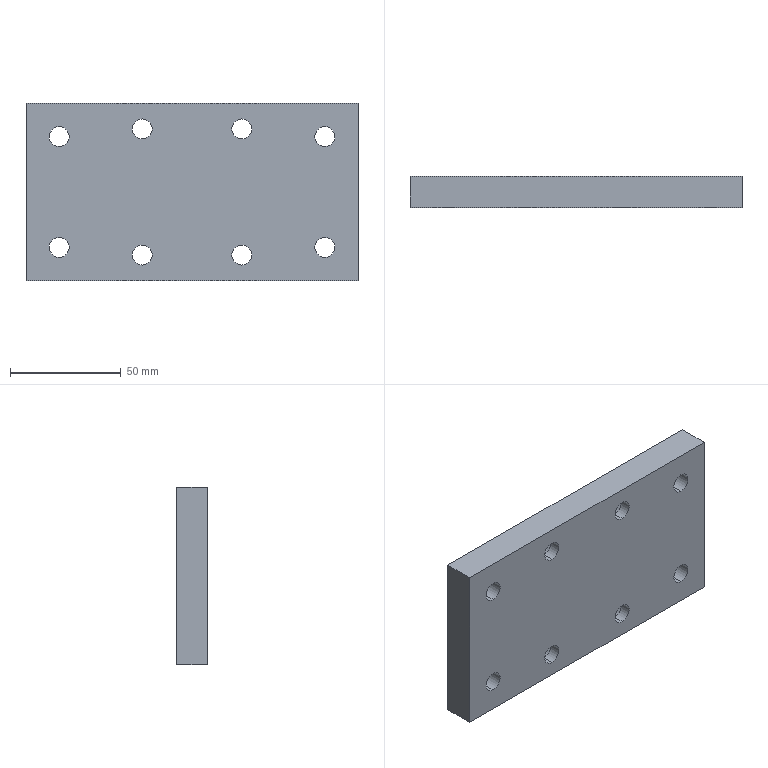Part | SolidWorks | features HoleWzd 2, Extrusion 1 | 1 solid | 34 faces | box 150 x 14 x 80 mm | volume 156803 mm3 | cylinder 24 | plane 10 | commonest cylinder face diameters 9 x16 15 x8
STEP:
#1=CARTESIAN_POINT('',(15.,0.,-69.5));
#2=VERTEX_POINT('',#1);
#3=CARTESIAN_POINT('',(15.,0.,-60.5));
#4=VERTEX_POINT('',#3);
#5=CARTESIAN_POINT('',(15.,0.,-65.));
#6=DIRECTION('',(0.,1.,0.));
#7=DIRECTION('',(0.,0.,1.));
#8=AXIS2_PLACEMENT_3D('',#5,#6,#7);
#9=CIRCLE('',#8,4.5);
#10=EDGE_CURVE('',#2,#4,#9,.T.);
#11=ORIENTED_EDGE('',*,*,#10,.F.);
#12=CARTESIAN_POINT('',(15.,14.,-69.5));
#13=VERTEX_POINT('',#12);
#14=CARTESIAN_POINT('',(15.,14.,-69.5));
#15=DIRECTION('',(0.,1.,0.));
#16=VECTOR('',#15,1000.);
#17=LINE('',#14,#16);
#18=EDGE_CURVE('',#2,#13,#17,.T.);
#19=ORIENTED_EDGE('',*,*,#18,.T.);
#20=CARTESIAN_POINT('',(15.,14.,-60.5));
#21=VERTEX_POINT('',#20);
#22=CARTESIAN_POINT('',(15.,14.,-65.));
#23=DIRECTION('',(0.,1.,0.));
#24=DIRECTION('',(0.,0.,1.));
#25=AXIS2_PLACEMENT_3D('',#22,#23,#24);
#26=CIRCLE('',#25,4.5);
#27=EDGE_CURVE('',#13,#21,#26,.T.);
#28=ORIENTED_EDGE('',*,*,#27,.T.);
#29=CARTESIAN_POINT('',(15.,14.,-60.5));
#30=DIRECTION('',(0.,1.,0.));
#31=VECTOR('',#30,1000.);
#32=LINE('',#29,#31);
#33=EDGE_CURVE('',#4,#21,#32,.T.);
#34=ORIENTED_EDGE('',*,*,#33,.F.);
#35=EDGE_LOOP('',(#11,#19,#28,#34));
#36=FACE_OUTER_BOUND('',#35,.T.);
#37=CARTESIAN_POINT('',(15.,14.,-65.));
#38=DIRECTION('',(0.,1.,0.));
#39=DIRECTION('',(0.,0.,1.));
#40=AXIS2_PLACEMENT_3D('',#37,#38,#39);
#41=CYLINDRICAL_SURFACE('',#40,4.5);
#42=ADVANCED_FACE('',(#36),#41,.F.);
#43=CARTESIAN_POINT('',(15.,0.,-19.5));
#44=VERTEX_POINT('',#43);
#45=CARTESIAN_POINT('',(15.,0.,-10.5));
#46=VERTEX_POINT('',#45);
#47=CARTESIAN_POINT('',(15.,0.,-15.));
#48=DIRECTION('',(0.,1.,0.));
#49=DIRECTION('',(0.,0.,1.));
#50=AXIS2_PLACEMENT_3D('',#47,#48,#49);
#51=CIRCLE('',#50,4.5);
#52=EDGE_CURVE('',#44,#46,#51,.T.);
#53=ORIENTED_EDGE('',*,*,#52,.F.);
#54=CARTESIAN_POINT('',(15.,14.,-19.5));
#55=VERTEX_POINT('',#54);
#56=CARTESIAN_POINT('',(15.,14.,-19.5));
#57=DIRECTION('',(0.,1.,0.));
#58=VECTOR('',#57,1000.);
#59=LINE('',#56,#58);
#60=EDGE_CURVE('',#44,#55,#59,.T.);
#61=ORIENTED_EDGE('',*,*,#60,.T.);
#62=CARTESIAN_POINT('',(15.,14.,-10.5));
#63=VERTEX_POINT('',#62);
#64=CARTESIAN_POINT('',(15.,14.,-15.));
#65=DIRECTION('',(0.,1.,0.));
#66=DIRECTION('',(0.,0.,1.));
#67=AXIS2_PLACEMENT_3D('',#64,#65,#66);
#68=CIRCLE('',#67,4.5);
#69=EDGE_CURVE('',#55,#63,#68,.T.);
#70=ORIENTED_EDGE('',*,*,#69,.T.);
#71=CARTESIAN_POINT('',(15.,14.,-10.5));
#72=DIRECTION('',(0.,1.,0.));
#73=VECTOR('',#72,1000.);
#74=LINE('',#71,#73);
#75=EDGE_CURVE('',#46,#63,#74,.T.);
#76=ORIENTED_EDGE('',*,*,#75,.F.);
#77=EDGE_LOOP('',(#53,#61,#70,#76));
#78=FACE_OUTER_BOUND('',#77,.T.);
#79=CARTESIAN_POINT('',(15.,14.,-15.));
#80=DIRECTION('',(0.,1.,0.));
#81=DIRECTION('',(0.,0.,1.));
#82=AXIS2_PLACEMENT_3D('',#79,#80,#81);
#83=CYLINDRICAL_SURFACE('',#82,4.5);
#84=ADVANCED_FACE('',(#78),#83,.F.);
#85=CARTESIAN_POINT('',(135.,0.,-19.5));
#86=VERTEX_POINT('',#85);
#87=CARTESIAN_POINT('',(135.,0.,-10.5));
#88=VERTEX_POINT('',#87);
#89=CARTESIAN_POINT('',(135.,0.,-15.));
#90=DIRECTION('',(0.,1.,0.));
#91=DIRECTION('',(0.,0.,1.));
#92=AXIS2_PLACEMENT_3D('',#89,#90,#91);
#93=CIRCLE('',#92,4.5);
#94=EDGE_CURVE('',#86,#88,#93,.T.);
#95=ORIENTED_EDGE('',*,*,#94,.F.);
#96=CARTESIAN_POINT('',(135.,14.,-19.5));
#97=VERTEX_POINT('',#96);
#98=CARTESIAN_POINT('',(135.,14.,-19.5));
#99=DIRECTION('',(0.,1.,0.));
#100=VECTOR('',#99,1000.);
#101=LINE('',#98,#100);
#102=EDGE_CURVE('',#86,#97,#101,.T.);
#103=ORIENTED_EDGE('',*,*,#102,.T.);
#104=CARTESIAN_POINT('',(135.,14.,-10.5));
#105=VERTEX_POINT('',#104);
#106=CARTESIAN_POINT('',(135.,14.,-15.));
#107=DIRECTION('',(0.,1.,0.));
#108=DIRECTION('',(0.,0.,1.));
#109=AXIS2_PLACEMENT_3D('',#106,#107,#108);
#110=CIRCLE('',#109,4.5);
#111=EDGE_CURVE('',#97,#105,#110,.T.);
#112=ORIENTED_EDGE('',*,*,#111,.T.);
#113=CARTESIAN_POINT('',(135.,14.,-10.5));
#114=DIRECTION('',(0.,1.,0.));
#115=VECTOR('',#114,1000.);
#116=LINE('',#113,#115);
#117=EDGE_CURVE('',#88,#105,#116,.T.);
#118=ORIENTED_EDGE('',*,*,#117,.F.);
#119=EDGE_LOOP('',(#95,#103,#112,#118));
#120=FACE_OUTER_BOUND('',#119,.T.);
#121=CARTESIAN_POINT('',(135.,14.,-15.));
#122=DIRECTION('',(0.,1.,0.));
#123=DIRECTION('',(0.,0.,1.));
#124=AXIS2_PLACEMENT_3D('',#121,#122,#123);
#125=CYLINDRICAL_SURFACE('',#124,4.5);
#126=ADVANCED_FACE('',(#120),#125,.F.);
#127=CARTESIAN_POINT('',(135.,0.,-69.5));
#128=VERTEX_POINT('',#127);
#129=CARTESIAN_POINT('',(135.,0.,-60.5));
#130=VERTEX_POINT('',#129);
#131=CARTESIAN_POINT('',(135.,0.,-65.));
#132=DIRECTION('',(0.,1.,0.));
#133=DIRECTION('',(0.,0.,1.));
#134=AXIS2_PLACEMENT_3D('',#131,#132,#133);
#135=CIRCLE('',#134,4.5);
#136=EDGE_CURVE('',#128,#130,#135,.T.);
#137=ORIENTED_EDGE('',*,*,#136,.F.);
#138=CARTESIAN_POINT('',(135.,14.,-69.5));
#139=VERTEX_POINT('',#138);
#140=CARTESIAN_POINT('',(135.,14.,-69.5));
#141=DIRECTION('',(0.,1.,0.));
#142=VECTOR('',#141,1000.);
#143=LINE('',#140,#142);
#144=EDGE_CURVE('',#128,#139,#143,.T.);
#145=ORIENTED_EDGE('',*,*,#144,.T.);
#146=CARTESIAN_POINT('',(135.,14.,-60.5));
#147=VERTEX_POINT('',#146);
#148=CARTESIAN_POINT('',(135.,14.,-65.));
#149=DIRECTION('',(0.,1.,0.));
#150=DIRECTION('',(0.,0.,1.));
#151=AXIS2_PLACEMENT_3D('',#148,#149,#150);
#152=CIRCLE('',#151,4.5);
#153=EDGE_CURVE('',#139,#147,#152,.T.);
#154=ORIENTED_EDGE('',*,*,#153,.T.);
#155=CARTESIAN_POINT('',(135.,14.,-60.5));
#156=DIRECTION('',(0.,1.,0.));
#157=VECTOR('',#156,1000.);
#158=LINE('',#155,#157);
#159=EDGE_CURVE('',#130,#147,#158,.T.);
#160=ORIENTED_EDGE('',*,*,#159,.F.);
#161=EDGE_LOOP('',(#137,#145,#154,#160));
#162=FACE_OUTER_BOUND('',#161,.T.);
#163=CARTESIAN_POINT('',(135.,14.,-65.));
#164=DIRECTION('',(0.,1.,0.));
#165=DIRECTION('',(0.,0.,1.));
#166=AXIS2_PLACEMENT_3D('',#163,#164,#165);
#167=CYLINDRICAL_SURFACE('',#166,4.5);
#168=ADVANCED_FACE('',(#162),#167,.F.);
#169=CARTESIAN_POINT('',(52.5,5.,-76.));
#170=VERTEX_POINT('',#169);
#171=CARTESIAN_POINT('',(52.5,5.,-61.));
#172=VERTEX_POINT('',#171);
#173=CARTESIAN_POINT('',(52.5,5.,-68.5));
#174=DIRECTION('',(0.,1.,0.));
#175=DIRECTION('',(0.,0.,1.));
#176=AXIS2_PLACEMENT_3D('',#173,#174,#175);
#177=CIRCLE('',#176,7.5);
#178=EDGE_CURVE('',#170,#172,#177,.T.);
#179=ORIENTED_EDGE('',*,*,#178,.F.);
#180=CARTESIAN_POINT('',(52.5,14.,-76.));
#181=VERTEX_POINT('',#180);
#182=CARTESIAN_POINT('',(52.5,14.,-76.));
#183=DIRECTION('',(0.,1.,0.));
#184=VECTOR('',#183,1000.);
#185=LINE('',#182,#184);
#186=EDGE_CURVE('',#170,#181,#185,.T.);
#187=ORIENTED_EDGE('',*,*,#186,.T.);
#188=CARTESIAN_POINT('',(52.5,14.,-61.));
#189=VERTEX_POINT('',#188);
#190=CARTESIAN_POINT('',(52.5,14.,-68.5));
#191=DIRECTION('',(0.,1.,0.));
#192=DIRECTION('',(0.,0.,1.));
#193=AXIS2_PLACEMENT_3D('',#190,#191,#192);
#194=CIRCLE('',#193,7.5);
#195=EDGE_CURVE('',#181,#189,#194,.T.);
#196=ORIENTED_EDGE('',*,*,#195,.T.);
#197=CARTESIAN_POINT('',(52.5,14.,-61.));
#198=DIRECTION('',(0.,1.,0.));
#199=VECTOR('',#198,1000.);
#200=LINE('',#197,#199);
#201=EDGE_CURVE('',#172,#189,#200,.T.);
#202=ORIENTED_EDGE('',*,*,#201,.F.);
#203=EDGE_LOOP('',(#179,#187,#196,#202));
#204=FACE_OUTER_BOUND('',#203,.T.);
#205=CARTESIAN_POINT('',(52.5,14.,-68.5));
#206=DIRECTION('',(0.,1.,0.));
#207=DIRECTION('',(0.,0.,1.));
#208=AXIS2_PLACEMENT_3D('',#205,#206,#207);
#209=CYLINDRICAL_SURFACE('',#208,7.5);
#210=ADVANCED_FACE('',(#204),#209,.F.);
#211=CARTESIAN_POINT('',(52.5,0.,-73.));
#212=VERTEX_POINT('',#211);
#213=CARTESIAN_POINT('',(52.5,0.,-64.));
#214=VERTEX_POINT('',#213);
#215=CARTESIAN_POINT('',(52.5,0.,-68.5));
#216=DIRECTION('',(0.,1.,0.));
#217=DIRECTION('',(0.,0.,1.));
#218=AXIS2_PLACEMENT_3D('',#215,#216,#217);
#219=CIRCLE('',#218,4.5);
#220=EDGE_CURVE('',#212,#214,#219,.T.);
#221=ORIENTED_EDGE('',*,*,#220,.F.);
#222=CARTESIAN_POINT('',(52.5,5.,-73.));
#223=VERTEX_POINT('',#222);
#224=CARTESIAN_POINT('',(52.5,14.,-73.));
#225=DIRECTION('',(0.,1.,0.));
#226=VECTOR('',#225,1000.);
#227=LINE('',#224,#226);
#228=EDGE_CURVE('',#212,#223,#227,.T.);
#229=ORIENTED_EDGE('',*,*,#228,.T.);
#230=CARTESIAN_POINT('',(52.5,5.,-64.));
#231=VERTEX_POINT('',#230);
#232=CARTESIAN_POINT('',(52.5,5.,-68.5));
#233=DIRECTION('',(0.,1.,0.));
#234=DIRECTION('',(0.,0.,1.));
#235=AXIS2_PLACEMENT_3D('',#232,#233,#234);
#236=CIRCLE('',#235,4.5);
#237=EDGE_CURVE('',#223,#231,#236,.T.);
#238=ORIENTED_EDGE('',*,*,#237,.T.);
#239=CARTESIAN_POINT('',(52.5,14.,-64.));
#240=DIRECTION('',(0.,1.,0.));
#241=VECTOR('',#240,1000.);
#242=LINE('',#239,#241);
#243=EDGE_CURVE('',#214,#231,#242,.T.);
#244=ORIENTED_EDGE('',*,*,#243,.F.);
#245=EDGE_LOOP('',(#221,#229,#238,#244));
#246=FACE_OUTER_BOUND('',#245,.T.);
#247=CARTESIAN_POINT('',(52.5,14.,-68.5));
#248=DIRECTION('',(0.,1.,0.));
#249=DIRECTION('',(0.,0.,1.));
#250=AXIS2_PLACEMENT_3D('',#247,#248,#249);
#251=CYLINDRICAL_SURFACE('',#250,4.5);
#252=ADVANCED_FACE('',(#246),#251,.F.);
#253=CARTESIAN_POINT('',(52.5,5.,-19.));
#254=VERTEX_POINT('',#253);
#255=CARTESIAN_POINT('',(52.5,5.,-4.));
#256=VERTEX_POINT('',#255);
#257=CARTESIAN_POINT('',(52.5,5.,-11.5));
#258=DIRECTION('',(0.,1.,0.));
#259=DIRECTION('',(0.,0.,1.));
#260=AXIS2_PLACEMENT_3D('',#257,#258,#259);
#261=CIRCLE('',#260,7.5);
#262=EDGE_CURVE('',#254,#256,#261,.T.);
#263=ORIENTED_EDGE('',*,*,#262,.F.);
#264=CARTESIAN_POINT('',(52.5,14.,-19.));
#265=VERTEX_POINT('',#264);
#266=CARTESIAN_POINT('',(52.5,14.,-19.));
#267=DIRECTION('',(0.,1.,0.));
#268=VECTOR('',#267,1000.);
#269=LINE('',#266,#268);
#270=EDGE_CURVE('',#254,#265,#269,.T.);
#271=ORIENTED_EDGE('',*,*,#270,.T.);
#272=CARTESIAN_POINT('',(52.5,14.,-4.));
#273=VERTEX_POINT('',#272);
#274=CARTESIAN_POINT('',(52.5,14.,-11.5));
#275=DIRECTION('',(0.,1.,0.));
#276=DIRECTION('',(0.,0.,1.));
#277=AXIS2_PLACEMENT_3D('',#274,#275,#276);
#278=CIRCLE('',#277,7.5);
#279=EDGE_CURVE('',#265,#273,#278,.T.);
#280=ORIENTED_EDGE('',*,*,#279,.T.);
#281=CARTESIAN_POINT('',(52.5,14.,-4.));
#282=DIRECTION('',(0.,1.,0.));
#283=VECTOR('',#282,1000.);
#284=LINE('',#281,#283);
#285=EDGE_CURVE('',#256,#273,#284,.T.);
#286=ORIENTED_EDGE('',*,*,#285,.F.);
#287=EDGE_LOOP('',(#263,#271,#280,#286));
#288=FACE_OUTER_BOUND('',#287,.T.);
#289=CARTESIAN_POINT('',(52.5,14.,-11.5));
#290=DIRECTION('',(0.,1.,0.));
#291=DIRECTION('',(0.,0.,1.));
#292=AXIS2_PLACEMENT_3D('',#289,#290,#291);
#293=CYLINDRICAL_SURFACE('',#292,7.5);
#294=ADVANCED_FACE('',(#288),#293,.F.);
#295=CARTESIAN_POINT('',(52.5,0.,-16.));
#296=VERTEX_POINT('',#295);
#297=CARTESIAN_POINT('',(52.5,0.,-7.));
#298=VERTEX_POINT('',#297);
#299=CARTESIAN_POINT('',(52.5,0.,-11.5));
#300=DIRECTION('',(0.,1.,0.));
#301=DIRECTION('',(0.,0.,1.));
#302=AXIS2_PLACEMENT_3D('',#299,#300,#301);
#303=CIRCLE('',#302,4.5);
#304=EDGE_CURVE('',#296,#298,#303,.T.);
#305=ORIENTED_EDGE('',*,*,#304,.F.);
#306=CARTESIAN_POINT('',(52.5,5.,-16.));
#307=VERTEX_POINT('',#306);
#308=CARTESIAN_POINT('',(52.5,14.,-16.));
#309=DIRECTION('',(0.,1.,0.));
#310=VECTOR('',#309,1000.);
#311=LINE('',#308,#310);
#312=EDGE_CURVE('',#296,#307,#311,.T.);
#313=ORIENTED_EDGE('',*,*,#312,.T.);
#314=CARTESIAN_POINT('',(52.5,5.,-7.));
#315=VERTEX_POINT('',#314);
#316=CARTESIAN_POINT('',(52.5,5.,-11.5));
#317=DIRECTION('',(0.,1.,0.));
#318=DIRECTION('',(0.,0.,1.));
#319=AXIS2_PLACEMENT_3D('',#316,#317,#318);
#320=CIRCLE('',#319,4.5);
#321=EDGE_CURVE('',#307,#315,#320,.T.);
#322=ORIENTED_EDGE('',*,*,#321,.T.);
#323=CARTESIAN_POINT('',(52.5,14.,-7.));
#324=DIRECTION('',(0.,1.,0.));
#325=VECTOR('',#324,1000.);
#326=LINE('',#323,#325);
#327=EDGE_CURVE('',#298,#315,#326,.T.);
#328=ORIENTED_EDGE('',*,*,#327,.F.);
#329=EDGE_LOOP('',(#305,#313,#322,#328));
#330=FACE_OUTER_BOUND('',#329,.T.);
#331=CARTESIAN_POINT('',(52.5,14.,-11.5));
#332=DIRECTION('',(0.,1.,0.));
#333=DIRECTION('',(0.,0.,1.));
#334=AXIS2_PLACEMENT_3D('',#331,#332,#333);
#335=CYLINDRICAL_SURFACE('',#334,4.5);
#336=ADVANCED_FACE('',(#330),#335,.F.);
#337=CARTESIAN_POINT('',(97.5,5.,-19.));
#338=VERTEX_POINT('',#337);
#339=CARTESIAN_POINT('',(97.5,5.,-4.));
#340=VERTEX_POINT('',#339);
#341=CARTESIAN_POINT('',(97.5,5.,-11.5));
#342=DIRECTION('',(0.,1.,0.));
#343=DIRECTION('',(0.,0.,1.));
#344=AXIS2_PLACEMENT_3D('',#341,#342,#343);
#345=CIRCLE('',#344,7.5);
#346=EDGE_CURVE('',#338,#340,#345,.T.);
#347=ORIENTED_EDGE('',*,*,#346,.F.);
#348=CARTESIAN_POINT('',(97.5,14.,-19.));
#349=VERTEX_POINT('',#348);
#350=CARTESIAN_POINT('',(97.5,14.,-19.));
#351=DIRECTION('',(0.,1.,0.));
#352=VECTOR('',#351,1000.);
#353=LINE('',#350,#352);
#354=EDGE_CURVE('',#338,#349,#353,.T.);
#355=ORIENTED_EDGE('',*,*,#354,.T.);
#356=CARTESIAN_POINT('',(97.5,14.,-4.));
#357=VERTEX_POINT('',#356);
#358=CARTESIAN_POINT('',(97.5,14.,-11.5));
#359=DIRECTION('',(0.,1.,0.));
#360=DIRECTION('',(0.,0.,1.));
#361=AXIS2_PLACEMENT_3D('',#358,#359,#360);
#362=CIRCLE('',#361,7.5);
#363=EDGE_CURVE('',#349,#357,#362,.T.);
#364=ORIENTED_EDGE('',*,*,#363,.T.);
#365=CARTESIAN_POINT('',(97.5,14.,-4.));
#366=DIRECTION('',(0.,1.,0.));
#367=VECTOR('',#366,1000.);
#368=LINE('',#365,#367);
#369=EDGE_CURVE('',#340,#357,#368,.T.);
#370=ORIENTED_EDGE('',*,*,#369,.F.);
#371=EDGE_LOOP('',(#347,#355,#364,#370));
#372=FACE_OUTER_BOUND('',#371,.T.);
#373=CARTESIAN_POINT('',(97.5,14.,-11.5));
#374=DIRECTION('',(0.,1.,0.));
#375=DIRECTION('',(0.,0.,1.));
#376=AXIS2_PLACEMENT_3D('',#373,#374,#375);
#377=CYLINDRICAL_SURFACE('',#376,7.5);
#378=ADVANCED_FACE('',(#372),#377,.F.);
#379=CARTESIAN_POINT('',(97.5,0.,-16.));
#380=VERTEX_POINT('',#379);
#381=CARTESIAN_POINT('',(97.5,0.,-7.));
#382=VERTEX_POINT('',#381);
#383=CARTESIAN_POINT('',(97.5,0.,-11.5));
#384=DIRECTION('',(0.,1.,0.));
#385=DIRECTION('',(0.,0.,1.));
#386=AXIS2_PLACEMENT_3D('',#383,#384,#385);
#387=CIRCLE('',#386,4.5);
#388=EDGE_CURVE('',#380,#382,#387,.T.);
#389=ORIENTED_EDGE('',*,*,#388,.F.);
#390=CARTESIAN_POINT('',(97.5,5.,-16.));
#391=VERTEX_POINT('',#390);
#392=CARTESIAN_POINT('',(97.5,14.,-16.));
#393=DIRECTION('',(0.,1.,0.));
#394=VECTOR('',#393,1000.);
#395=LINE('',#392,#394);
#396=EDGE_CURVE('',#380,#391,#395,.T.);
#397=ORIENTED_EDGE('',*,*,#396,.T.);
#398=CARTESIAN_POINT('',(97.5,5.,-7.));
#399=VERTEX_POINT('',#398);
#400=CARTESIAN_POINT('',(97.5,5.,-11.5));
#401=DIRECTION('',(0.,1.,0.));
#402=DIRECTION('',(0.,0.,1.));
#403=AXIS2_PLACEMENT_3D('',#400,#401,#402);
#404=CIRCLE('',#403,4.5);
#405=EDGE_CURVE('',#391,#399,#404,.T.);
#406=ORIENTED_EDGE('',*,*,#405,.T.);
#407=CARTESIAN_POINT('',(97.5,14.,-7.));
#408=DIRECTION('',(0.,1.,0.));
#409=VECTOR('',#408,1000.);
#410=LINE('',#407,#409);
#411=EDGE_CURVE('',#382,#399,#410,.T.);
#412=ORIENTED_EDGE('',*,*,#411,.F.);
#413=EDGE_LOOP('',(#389,#397,#406,#412));
#414=FACE_OUTER_BOUND('',#413,.T.);
#415=CARTESIAN_POINT('',(97.5,14.,-11.5));
#416=DIRECTION('',(0.,1.,0.));
#417=DIRECTION('',(0.,0.,1.));
#418=AXIS2_PLACEMENT_3D('',#415,#416,#417);
#419=CYLINDRICAL_SURFACE('',#418,4.5);
#420=ADVANCED_FACE('',(#414),#419,.F.);
#421=CARTESIAN_POINT('',(97.5,5.,-76.));
#422=VERTEX_POINT('',#421);
#423=CARTESIAN_POINT('',(97.5,5.,-61.));
#424=VERTEX_POINT('',#423);
#425=CARTESIAN_POINT('',(97.5,5.,-68.5));
#426=DIRECTION('',(0.,1.,0.));
#427=DIRECTION('',(0.,0.,1.));
#428=AXIS2_PLACEMENT_3D('',#425,#426,#427);
#429=CIRCLE('',#428,7.5);
#430=EDGE_CURVE('',#422,#424,#429,.T.);
#431=ORIENTED_EDGE('',*,*,#430,.F.);
#432=CARTESIAN_POINT('',(97.5,14.,-76.));
#433=VERTEX_POINT('',#432);
#434=CARTESIAN_POINT('',(97.5,14.,-76.));
#435=DIRECTION('',(0.,1.,0.));
#436=VECTOR('',#435,1000.);
#437=LINE('',#434,#436);
#438=EDGE_CURVE('',#422,#433,#437,.T.);
#439=ORIENTED_EDGE('',*,*,#438,.T.);
#440=CARTESIAN_POINT('',(97.5,14.,-61.));
#441=VERTEX_POINT('',#440);
#442=CARTESIAN_POINT('',(97.5,14.,-68.5));
#443=DIRECTION('',(0.,1.,0.));
#444=DIRECTION('',(0.,0.,1.));
#445=AXIS2_PLACEMENT_3D('',#442,#443,#444);
#446=CIRCLE('',#445,7.5);
#447=EDGE_CURVE('',#433,#441,#446,.T.);
#448=ORIENTED_EDGE('',*,*,#447,.T.);
#449=CARTESIAN_POINT('',(97.5,14.,-61.));
#450=DIRECTION('',(0.,1.,0.));
#451=VECTOR('',#450,1000.);
#452=LINE('',#449,#451);
#453=EDGE_CURVE('',#424,#441,#452,.T.);
#454=ORIENTED_EDGE('',*,*,#453,.F.);
#455=EDGE_LOOP('',(#431,#439,#448,#454));
#456=FACE_OUTER_BOUND('',#455,.T.);
#457=CARTESIAN_POINT('',(97.5,14.,-68.5));
#458=DIRECTION('',(0.,1.,0.));
#459=DIRECTION('',(0.,0.,1.));
#460=AXIS2_PLACEMENT_3D('',#457,#458,#459);
#461=CYLINDRICAL_SURFACE('',#460,7.5);
#462=ADVANCED_FACE('',(#456),#461,.F.);
#463=CARTESIAN_POINT('',(97.5,0.,-73.));
#464=VERTEX_POINT('',#463);
#465=CARTESIAN_POINT('',(97.5,0.,-64.));
#466=VERTEX_POINT('',#465);
#467=CARTESIAN_POINT('',(97.5,0.,-68.5));
#468=DIRECTION('',(0.,1.,0.));
#469=DIRECTION('',(0.,0.,1.));
#470=AXIS2_PLACEMENT_3D('',#467,#468,#469);
#471=CIRCLE('',#470,4.5);
#472=EDGE_CURVE('',#464,#466,#471,.T.);
#473=ORIENTED_EDGE('',*,*,#472,.F.);
#474=CARTESIAN_POINT('',(97.5,5.,-73.));
#475=VERTEX_POINT('',#474);
#476=CARTESIAN_POINT('',(97.5,14.,-73.));
#477=DIRECTION('',(0.,1.,0.));
#478=VECTOR('',#477,1000.);
#479=LINE('',#476,#478);
#480=EDGE_CURVE('',#464,#475,#479,.T.);
#481=ORIENTED_EDGE('',*,*,#480,.T.);
#482=CARTESIAN_POINT('',(97.5,5.,-64.));
#483=VERTEX_POINT('',#482);
#484=CARTESIAN_POINT('',(97.5,5.,-68.5));
#485=DIRECTION('',(0.,1.,0.));
#486=DIRECTION('',(0.,0.,1.));
#487=AXIS2_PLACEMENT_3D('',#484,#485,#486);
#488=CIRCLE('',#487,4.5);
#489=EDGE_CURVE('',#475,#483,#488,.T.);
#490=ORIENTED_EDGE('',*,*,#489,.T.);
#491=CARTESIAN_POINT('',(97.5,14.,-64.));
#492=DIRECTION('',(0.,1.,0.));
#493=VECTOR('',#492,1000.);
#494=LINE('',#491,#493);
#495=EDGE_CURVE('',#466,#483,#494,.T.);
#496=ORIENTED_EDGE('',*,*,#495,.F.);
#497=EDGE_LOOP('',(#473,#481,#490,#496));
#498=FACE_OUTER_BOUND('',#497,.T.);
#499=CARTESIAN_POINT('',(97.5,14.,-68.5));
#500=DIRECTION('',(0.,1.,0.));
#501=DIRECTION('',(0.,0.,1.));
#502=AXIS2_PLACEMENT_3D('',#499,#500,#501);
#503=CYLINDRICAL_SURFACE('',#502,4.5);
#504=ADVANCED_FACE('',(#498),#503,.F.);
#505=CARTESIAN_POINT('',(0.,0.,-80.));
#506=VERTEX_POINT('',#505);
#507=CARTESIAN_POINT('',(0.,0.,0.));
#508=VERTEX_POINT('',#507);
#509=CARTESIAN_POINT('',(0.,0.,0.));
#510=DIRECTION('',(0.,0.,1.));
#511=VECTOR('',#510,1000.);
#512=LINE('',#509,#511);
#513=EDGE_CURVE('',#506,#508,#512,.T.);
#514=ORIENTED_EDGE('',*,*,#513,.T.);
#515=CARTESIAN_POINT('',(0.,14.,0.));
#516=VERTEX_POINT('',#515);
#517=CARTESIAN_POINT('',(0.,14.,0.));
#518=DIRECTION('',(0.,-1.,0.));
#519=VECTOR('',#518,1000.);
#520=LINE('',#517,#519);
#521=EDGE_CURVE('',#516,#508,#520,.T.);
#522=ORIENTED_EDGE('',*,*,#521,.F.);
#523=CARTESIAN_POINT('',(0.,14.,-80.));
#524=VERTEX_POINT('',#523);
#525=CARTESIAN_POINT('',(0.,14.,0.));
#526=DIRECTION('',(0.,0.,1.));
#527=VECTOR('',#526,1000.);
#528=LINE('',#525,#527);
#529=EDGE_CURVE('',#524,#516,#528,.T.);
#530=ORIENTED_EDGE('',*,*,#529,.F.);
#531=CARTESIAN_POINT('',(0.,14.,-80.));
#532=DIRECTION('',(0.,-1.,0.));
#533=VECTOR('',#532,1000.);
#534=LINE('',#531,#533);
#535=EDGE_CURVE('',#524,#506,#534,.T.);
#536=ORIENTED_EDGE('',*,*,#535,.T.);
#537=EDGE_LOOP('',(#514,#522,#530,#536));
#538=FACE_OUTER_BOUND('',#537,.T.);
#539=CARTESIAN_POINT('',(0.,14.,0.));
#540=DIRECTION('',(1.,0.,0.));
#541=DIRECTION('',(0.,0.,-1.));
#542=AXIS2_PLACEMENT_3D('',#539,#540,#541);
#543=PLANE('',#542);
#544=ADVANCED_FACE('',(#538),#543,.F.);
#545=CARTESIAN_POINT('',(150.,0.,0.));
#546=VERTEX_POINT('',#545);
#547=CARTESIAN_POINT('',(0.,0.,0.));
#548=DIRECTION('',(1.,0.,0.));
#549=VECTOR('',#548,1000.);
#550=LINE('',#547,#549);
#551=EDGE_CURVE('',#508,#546,#550,.T.);
#552=ORIENTED_EDGE('',*,*,#551,.T.);
#553=CARTESIAN_POINT('',(150.,14.,0.));
#554=VERTEX_POINT('',#553);
#555=CARTESIAN_POINT('',(150.,14.,0.));
#556=DIRECTION('',(0.,-1.,0.));
#557=VECTOR('',#556,1000.);
#558=LINE('',#555,#557);
#559=EDGE_CURVE('',#554,#546,#558,.T.);
#560=ORIENTED_EDGE('',*,*,#559,.F.);
#561=CARTESIAN_POINT('',(0.,14.,0.));
#562=DIRECTION('',(1.,0.,0.));
#563=VECTOR('',#562,1000.);
#564=LINE('',#561,#563);
#565=EDGE_CURVE('',#516,#554,#564,.T.);
#566=ORIENTED_EDGE('',*,*,#565,.F.);
#567=ORIENTED_EDGE('',*,*,#521,.T.);
#568=EDGE_LOOP('',(#552,#560,#566,#567));
#569=FACE_OUTER_BOUND('',#568,.T.);
#570=CARTESIAN_POINT('',(0.,14.,0.));
#571=DIRECTION('',(0.,0.,-1.));
#572=DIRECTION('',(-1.,0.,0.));
#573=AXIS2_PLACEMENT_3D('',#570,#571,#572);
#574=PLANE('',#573);
#575=ADVANCED_FACE('',(#569),#574,.F.);
#576=CARTESIAN_POINT('',(150.,0.,-80.));
#577=VERTEX_POINT('',#576);
#578=CARTESIAN_POINT('',(150.,0.,0.));
#579=DIRECTION('',(0.,0.,-1.));
#580=VECTOR('',#579,1000.);
#581=LINE('',#578,#580);
#582=EDGE_CURVE('',#546,#577,#581,.T.);
#583=ORIENTED_EDGE('',*,*,#582,.T.);
#584=CARTESIAN_POINT('',(150.,14.,-80.));
#585=VERTEX_POINT('',#584);
#586=CARTESIAN_POINT('',(150.,14.,-80.));
#587=DIRECTION('',(0.,-1.,0.));
#588=VECTOR('',#587,1000.);
#589=LINE('',#586,#588);
#590=EDGE_CURVE('',#585,#577,#589,.T.);
#591=ORIENTED_EDGE('',*,*,#590,.F.);
#592=CARTESIAN_POINT('',(150.,14.,0.));
#593=DIRECTION('',(0.,0.,-1.));
#594=VECTOR('',#593,1000.);
#595=LINE('',#592,#594);
#596=EDGE_CURVE('',#554,#585,#595,.T.);
#597=ORIENTED_EDGE('',*,*,#596,.F.);
#598=ORIENTED_EDGE('',*,*,#559,.T.);
#599=EDGE_LOOP('',(#583,#591,#597,#598));
#600=FACE_OUTER_BOUND('',#599,.T.);
#601=CARTESIAN_POINT('',(150.,14.,0.));
#602=DIRECTION('',(-1.,0.,0.));
#603=DIRECTION('',(0.,0.,1.));
#604=AXIS2_PLACEMENT_3D('',#601,#602,#603);
#605=PLANE('',#604);
#606=ADVANCED_FACE('',(#600),#605,.F.);
#607=CARTESIAN_POINT('',(0.,0.,-80.));
#608=DIRECTION('',(-1.,0.,0.));
#609=VECTOR('',#608,1000.);
#610=LINE('',#607,#609);
#611=EDGE_CURVE('',#577,#506,#610,.T.);
#612=ORIENTED_EDGE('',*,*,#611,.T.);
#613=ORIENTED_EDGE('',*,*,#535,.F.);
#614=CARTESIAN_POINT('',(0.,14.,-80.));
#615=DIRECTION('',(-1.,0.,0.));
#616=VECTOR('',#615,1000.);
#617=LINE('',#614,#616);
#618=EDGE_CURVE('',#585,#524,#617,.T.);
#619=ORIENTED_EDGE('',*,*,#618,.F.);
#620=ORIENTED_EDGE('',*,*,#590,.T.);
#621=EDGE_LOOP('',(#612,#613,#619,#620));
#622=FACE_OUTER_BOUND('',#621,.T.);
#623=CARTESIAN_POINT('',(0.,14.,-80.));
#624=DIRECTION('',(0.,0.,1.));
#625=DIRECTION('',(1.,0.,0.));
#626=AXIS2_PLACEMENT_3D('',#623,#624,#625);
#627=PLANE('',#626);
#628=ADVANCED_FACE('',(#622),#627,.F.);
#629=CARTESIAN_POINT('',(15.,14.,-65.));
#630=DIRECTION('',(0.,1.,0.));
#631=DIRECTION('',(0.,0.,1.));
#632=AXIS2_PLACEMENT_3D('',#629,#630,#631);
#633=CIRCLE('',#632,4.5);
#634=EDGE_CURVE('',#21,#13,#633,.T.);
#635=ORIENTED_EDGE('',*,*,#634,.F.);
#636=ORIENTED_EDGE('',*,*,#27,.F.);
#637=EDGE_LOOP('',(#635,#636));
#638=FACE_BOUND('',#637,.T.);
#639=CARTESIAN_POINT('',(15.,14.,-15.));
#640=DIRECTION('',(0.,1.,0.));
#641=DIRECTION('',(0.,0.,1.));
#642=AXIS2_PLACEMENT_3D('',#639,#640,#641);
#643=CIRCLE('',#642,4.5);
#644=EDGE_CURVE('',#63,#55,#643,.T.);
#645=ORIENTED_EDGE('',*,*,#644,.F.);
#646=ORIENTED_EDGE('',*,*,#69,.F.);
#647=EDGE_LOOP('',(#645,#646));
#648=FACE_BOUND('',#647,.T.);
#649=CARTESIAN_POINT('',(135.,14.,-15.));
#650=DIRECTION('',(0.,1.,0.));
#651=DIRECTION('',(0.,0.,1.));
#652=AXIS2_PLACEMENT_3D('',#649,#650,#651);
#653=CIRCLE('',#652,4.5);
#654=EDGE_CURVE('',#105,#97,#653,.T.);
#655=ORIENTED_EDGE('',*,*,#654,.F.);
#656=ORIENTED_EDGE('',*,*,#111,.F.);
#657=EDGE_LOOP('',(#655,#656));
#658=FACE_BOUND('',#657,.T.);
#659=CARTESIAN_POINT('',(135.,14.,-65.));
#660=DIRECTION('',(0.,1.,0.));
#661=DIRECTION('',(0.,0.,1.));
#662=AXIS2_PLACEMENT_3D('',#659,#660,#661);
#663=CIRCLE('',#662,4.5);
#664=EDGE_CURVE('',#147,#139,#663,.T.);
#665=ORIENTED_EDGE('',*,*,#664,.F.);
#666=ORIENTED_EDGE('',*,*,#153,.F.);
#667=EDGE_LOOP('',(#665,#666));
#668=FACE_BOUND('',#667,.T.);
#669=CARTESIAN_POINT('',(52.5,14.,-68.5));
#670=DIRECTION('',(0.,1.,0.));
#671=DIRECTION('',(0.,0.,1.));
#672=AXIS2_PLACEMENT_3D('',#669,#670,#671);
#673=CIRCLE('',#672,7.5);
#674=EDGE_CURVE('',#189,#181,#673,.T.);
#675=ORIENTED_EDGE('',*,*,#674,.F.);
#676=ORIENTED_EDGE('',*,*,#195,.F.);
#677=EDGE_LOOP('',(#675,#676));
#678=FACE_BOUND('',#677,.T.);
#679=CARTESIAN_POINT('',(52.5,14.,-11.5));
#680=DIRECTION('',(0.,1.,0.));
#681=DIRECTION('',(0.,0.,1.));
#682=AXIS2_PLACEMENT_3D('',#679,#680,#681);
#683=CIRCLE('',#682,7.5);
#684=EDGE_CURVE('',#273,#265,#683,.T.);
#685=ORIENTED_EDGE('',*,*,#684,.F.);
#686=ORIENTED_EDGE('',*,*,#279,.F.);
#687=EDGE_LOOP('',(#685,#686));
#688=FACE_BOUND('',#687,.T.);
#689=CARTESIAN_POINT('',(97.5,14.,-11.5));
#690=DIRECTION('',(0.,1.,0.));
#691=DIRECTION('',(0.,0.,1.));
#692=AXIS2_PLACEMENT_3D('',#689,#690,#691);
#693=CIRCLE('',#692,7.5);
#694=EDGE_CURVE('',#357,#349,#693,.T.);
#695=ORIENTED_EDGE('',*,*,#694,.F.);
#696=ORIENTED_EDGE('',*,*,#363,.F.);
#697=EDGE_LOOP('',(#695,#696));
#698=FACE_BOUND('',#697,.T.);
#699=CARTESIAN_POINT('',(97.5,14.,-68.5));
#700=DIRECTION('',(0.,1.,0.));
#701=DIRECTION('',(0.,0.,1.));
#702=AXIS2_PLACEMENT_3D('',#699,#700,#701);
#703=CIRCLE('',#702,7.5);
#704=EDGE_CURVE('',#441,#433,#703,.T.);
#705=ORIENTED_EDGE('',*,*,#704,.F.);
#706=ORIENTED_EDGE('',*,*,#447,.F.);
#707=EDGE_LOOP('',(#705,#706));
#708=FACE_BOUND('',#707,.T.);
#709=ORIENTED_EDGE('',*,*,#529,.T.);
#710=ORIENTED_EDGE('',*,*,#565,.T.);
#711=ORIENTED_EDGE('',*,*,#596,.T.);
#712=ORIENTED_EDGE('',*,*,#618,.T.);
#713=EDGE_LOOP('',(#709,#710,#711,#712));
#714=FACE_OUTER_BOUND('',#713,.T.);
#715=CARTESIAN_POINT('',(0.,14.,0.));
#716=DIRECTION('',(0.,-1.,0.));
#717=DIRECTION('',(0.,0.,-1.));
#718=AXIS2_PLACEMENT_3D('',#715,#716,#717);
#719=PLANE('',#718);
#720=ADVANCED_FACE('',(#638,#648,#658,#668,#678,#688,#698,#708,#714),#719,.F.);
#721=CARTESIAN_POINT('',(15.,0.,-65.));
#722=DIRECTION('',(0.,1.,0.));
#723=DIRECTION('',(0.,0.,1.));
#724=AXIS2_PLACEMENT_3D('',#721,#722,#723);
#725=CIRCLE('',#724,4.5);
#726=EDGE_CURVE('',#4,#2,#725,.T.);
#727=ORIENTED_EDGE('',*,*,#726,.T.);
#728=ORIENTED_EDGE('',*,*,#10,.T.);
#729=EDGE_LOOP('',(#727,#728));
#730=FACE_BOUND('',#729,.T.);
#731=CARTESIAN_POINT('',(15.,0.,-15.));
#732=DIRECTION('',(0.,1.,0.));
#733=DIRECTION('',(0.,0.,1.));
#734=AXIS2_PLACEMENT_3D('',#731,#732,#733);
#735=CIRCLE('',#734,4.5);
#736=EDGE_CURVE('',#46,#44,#735,.T.);
#737=ORIENTED_EDGE('',*,*,#736,.T.);
#738=ORIENTED_EDGE('',*,*,#52,.T.);
#739=EDGE_LOOP('',(#737,#738));
#740=FACE_BOUND('',#739,.T.);
#741=CARTESIAN_POINT('',(135.,0.,-15.));
#742=DIRECTION('',(0.,1.,0.));
#743=DIRECTION('',(0.,0.,1.));
#744=AXIS2_PLACEMENT_3D('',#741,#742,#743);
#745=CIRCLE('',#744,4.5);
#746=EDGE_CURVE('',#88,#86,#745,.T.);
#747=ORIENTED_EDGE('',*,*,#746,.T.);
#748=ORIENTED_EDGE('',*,*,#94,.T.);
#749=EDGE_LOOP('',(#747,#748));
#750=FACE_BOUND('',#749,.T.);
#751=CARTESIAN_POINT('',(135.,0.,-65.));
#752=DIRECTION('',(0.,1.,0.));
#753=DIRECTION('',(0.,0.,1.));
#754=AXIS2_PLACEMENT_3D('',#751,#752,#753);
#755=CIRCLE('',#754,4.5);
#756=EDGE_CURVE('',#130,#128,#755,.T.);
#757=ORIENTED_EDGE('',*,*,#756,.T.);
#758=ORIENTED_EDGE('',*,*,#136,.T.);
#759=EDGE_LOOP('',(#757,#758));
#760=FACE_BOUND('',#759,.T.);
#761=CARTESIAN_POINT('',(52.5,0.,-68.5));
#762=DIRECTION('',(0.,1.,0.));
#763=DIRECTION('',(0.,0.,1.));
#764=AXIS2_PLACEMENT_3D('',#761,#762,#763);
#765=CIRCLE('',#764,4.5);
#766=EDGE_CURVE('',#214,#212,#765,.T.);
#767=ORIENTED_EDGE('',*,*,#766,.T.);
#768=ORIENTED_EDGE('',*,*,#220,.T.);
#769=EDGE_LOOP('',(#767,#768));
#770=FACE_BOUND('',#769,.T.);
#771=CARTESIAN_POINT('',(52.5,0.,-11.5));
#772=DIRECTION('',(0.,1.,0.));
#773=DIRECTION('',(0.,0.,1.));
#774=AXIS2_PLACEMENT_3D('',#771,#772,#773);
#775=CIRCLE('',#774,4.5);
#776=EDGE_CURVE('',#298,#296,#775,.T.);
#777=ORIENTED_EDGE('',*,*,#776,.T.);
#778=ORIENTED_EDGE('',*,*,#304,.T.);
#779=EDGE_LOOP('',(#777,#778));
#780=FACE_BOUND('',#779,.T.);
#781=CARTESIAN_POINT('',(97.5,0.,-11.5));
#782=DIRECTION('',(0.,1.,0.));
#783=DIRECTION('',(0.,0.,1.));
#784=AXIS2_PLACEMENT_3D('',#781,#782,#783);
#785=CIRCLE('',#784,4.5);
#786=EDGE_CURVE('',#382,#380,#785,.T.);
#787=ORIENTED_EDGE('',*,*,#786,.T.);
#788=ORIENTED_EDGE('',*,*,#388,.T.);
#789=EDGE_LOOP('',(#787,#788));
#790=FACE_BOUND('',#789,.T.);
#791=CARTESIAN_POINT('',(97.5,0.,-68.5));
#792=DIRECTION('',(0.,1.,0.));
#793=DIRECTION('',(0.,0.,1.));
#794=AXIS2_PLACEMENT_3D('',#791,#792,#793);
#795=CIRCLE('',#794,4.5);
#796=EDGE_CURVE('',#466,#464,#795,.T.);
#797=ORIENTED_EDGE('',*,*,#796,.T.);
#798=ORIENTED_EDGE('',*,*,#472,.T.);
#799=EDGE_LOOP('',(#797,#798));
#800=FACE_BOUND('',#799,.T.);
#801=ORIENTED_EDGE('',*,*,#513,.F.);
#802=ORIENTED_EDGE('',*,*,#611,.F.);
#803=ORIENTED_EDGE('',*,*,#582,.F.);
#804=ORIENTED_EDGE('',*,*,#551,.F.);
#805=EDGE_LOOP('',(#801,#802,#803,#804));
#806=FACE_OUTER_BOUND('',#805,.T.);
#807=CARTESIAN_POINT('',(0.,0.,0.));
#808=DIRECTION('',(0.,-1.,0.));
#809=DIRECTION('',(0.,0.,-1.));
#810=AXIS2_PLACEMENT_3D('',#807,#808,#809);
#811=PLANE('',#810);
#812=ADVANCED_FACE('',(#730,#740,#750,#760,#770,#780,#790,#800,#806),#811,.T.);
#813=ORIENTED_EDGE('',*,*,#480,.F.);
#814=ORIENTED_EDGE('',*,*,#796,.F.);
#815=ORIENTED_EDGE('',*,*,#495,.T.);
#816=CARTESIAN_POINT('',(97.5,5.,-68.5));
#817=DIRECTION('',(0.,1.,0.));
#818=DIRECTION('',(0.,0.,1.));
#819=AXIS2_PLACEMENT_3D('',#816,#817,#818);
#820=CIRCLE('',#819,4.5);
#821=EDGE_CURVE('',#483,#475,#820,.T.);
#822=ORIENTED_EDGE('',*,*,#821,.T.);
#823=EDGE_LOOP('',(#813,#814,#815,#822));
#824=FACE_OUTER_BOUND('',#823,.T.);
#825=CARTESIAN_POINT('',(97.5,14.,-68.5));
#826=DIRECTION('',(0.,1.,0.));
#827=DIRECTION('',(0.,0.,1.));
#828=AXIS2_PLACEMENT_3D('',#825,#826,#827);
#829=CYLINDRICAL_SURFACE('',#828,4.5);
#830=ADVANCED_FACE('',(#824),#829,.F.);
#831=ORIENTED_EDGE('',*,*,#821,.F.);
#832=ORIENTED_EDGE('',*,*,#489,.F.);
#833=EDGE_LOOP('',(#831,#832));
#834=FACE_BOUND('',#833,.T.);
#835=CARTESIAN_POINT('',(97.5,5.,-68.5));
#836=DIRECTION('',(0.,1.,0.));
#837=DIRECTION('',(0.,0.,1.));
#838=AXIS2_PLACEMENT_3D('',#835,#836,#837);
#839=CIRCLE('',#838,7.5);
#840=EDGE_CURVE('',#424,#422,#839,.T.);
#841=ORIENTED_EDGE('',*,*,#840,.T.);
#842=ORIENTED_EDGE('',*,*,#430,.T.);
#843=EDGE_LOOP('',(#841,#842));
#844=FACE_OUTER_BOUND('',#843,.T.);
#845=CARTESIAN_POINT('',(102.,5.,-68.5));
#846=DIRECTION('',(0.,-1.,0.));
#847=DIRECTION('',(0.,0.,-1.));
#848=AXIS2_PLACEMENT_3D('',#845,#846,#847);
#849=PLANE('',#848);
#850=ADVANCED_FACE('',(#834,#844),#849,.F.);
#851=ORIENTED_EDGE('',*,*,#438,.F.);
#852=ORIENTED_EDGE('',*,*,#840,.F.);
#853=ORIENTED_EDGE('',*,*,#453,.T.);
#854=ORIENTED_EDGE('',*,*,#704,.T.);
#855=EDGE_LOOP('',(#851,#852,#853,#854));
#856=FACE_OUTER_BOUND('',#855,.T.);
#857=CARTESIAN_POINT('',(97.5,14.,-68.5));
#858=DIRECTION('',(0.,1.,0.));
#859=DIRECTION('',(0.,0.,1.));
#860=AXIS2_PLACEMENT_3D('',#857,#858,#859);
#861=CYLINDRICAL_SURFACE('',#860,7.5);
#862=ADVANCED_FACE('',(#856),#861,.F.);
#863=ORIENTED_EDGE('',*,*,#396,.F.);
#864=ORIENTED_EDGE('',*,*,#786,.F.);
#865=ORIENTED_EDGE('',*,*,#411,.T.);
#866=CARTESIAN_POINT('',(97.5,5.,-11.5));
#867=DIRECTION('',(0.,1.,0.));
#868=DIRECTION('',(0.,0.,1.));
#869=AXIS2_PLACEMENT_3D('',#866,#867,#868);
#870=CIRCLE('',#869,4.5);
#871=EDGE_CURVE('',#399,#391,#870,.T.);
#872=ORIENTED_EDGE('',*,*,#871,.T.);
#873=EDGE_LOOP('',(#863,#864,#865,#872));
#874=FACE_OUTER_BOUND('',#873,.T.);
#875=CARTESIAN_POINT('',(97.5,14.,-11.5));
#876=DIRECTION('',(0.,1.,0.));
#877=DIRECTION('',(0.,0.,1.));
#878=AXIS2_PLACEMENT_3D('',#875,#876,#877);
#879=CYLINDRICAL_SURFACE('',#878,4.5);
#880=ADVANCED_FACE('',(#874),#879,.F.);
#881=ORIENTED_EDGE('',*,*,#871,.F.);
#882=ORIENTED_EDGE('',*,*,#405,.F.);
#883=EDGE_LOOP('',(#881,#882));
#884=FACE_BOUND('',#883,.T.);
#885=CARTESIAN_POINT('',(97.5,5.,-11.5));
#886=DIRECTION('',(0.,1.,0.));
#887=DIRECTION('',(0.,0.,1.));
#888=AXIS2_PLACEMENT_3D('',#885,#886,#887);
#889=CIRCLE('',#888,7.5);
#890=EDGE_CURVE('',#340,#338,#889,.T.);
#891=ORIENTED_EDGE('',*,*,#890,.T.);
#892=ORIENTED_EDGE('',*,*,#346,.T.);
#893=EDGE_LOOP('',(#891,#892));
#894=FACE_OUTER_BOUND('',#893,.T.);
#895=CARTESIAN_POINT('',(102.,5.,-11.5));
#896=DIRECTION('',(0.,-1.,0.));
#897=DIRECTION('',(0.,0.,-1.));
#898=AXIS2_PLACEMENT_3D('',#895,#896,#897);
#899=PLANE('',#898);
#900=ADVANCED_FACE('',(#884,#894),#899,.F.);
#901=ORIENTED_EDGE('',*,*,#354,.F.);
#902=ORIENTED_EDGE('',*,*,#890,.F.);
#903=ORIENTED_EDGE('',*,*,#369,.T.);
#904=ORIENTED_EDGE('',*,*,#694,.T.);
#905=EDGE_LOOP('',(#901,#902,#903,#904));
#906=FACE_OUTER_BOUND('',#905,.T.);
#907=CARTESIAN_POINT('',(97.5,14.,-11.5));
#908=DIRECTION('',(0.,1.,0.));
#909=DIRECTION('',(0.,0.,1.));
#910=AXIS2_PLACEMENT_3D('',#907,#908,#909);
#911=CYLINDRICAL_SURFACE('',#910,7.5);
#912=ADVANCED_FACE('',(#906),#911,.F.);
#913=ORIENTED_EDGE('',*,*,#312,.F.);
#914=ORIENTED_EDGE('',*,*,#776,.F.);
#915=ORIENTED_EDGE('',*,*,#327,.T.);
#916=CARTESIAN_POINT('',(52.5,5.,-11.5));
#917=DIRECTION('',(0.,1.,0.));
#918=DIRECTION('',(0.,0.,1.));
#919=AXIS2_PLACEMENT_3D('',#916,#917,#918);
#920=CIRCLE('',#919,4.5);
#921=EDGE_CURVE('',#315,#307,#920,.T.);
#922=ORIENTED_EDGE('',*,*,#921,.T.);
#923=EDGE_LOOP('',(#913,#914,#915,#922));
#924=FACE_OUTER_BOUND('',#923,.T.);
#925=CARTESIAN_POINT('',(52.5,14.,-11.5));
#926=DIRECTION('',(0.,1.,0.));
#927=DIRECTION('',(0.,0.,1.));
#928=AXIS2_PLACEMENT_3D('',#925,#926,#927);
#929=CYLINDRICAL_SURFACE('',#928,4.5);
#930=ADVANCED_FACE('',(#924),#929,.F.);
#931=ORIENTED_EDGE('',*,*,#921,.F.);
#932=ORIENTED_EDGE('',*,*,#321,.F.);
#933=EDGE_LOOP('',(#931,#932));
#934=FACE_BOUND('',#933,.T.);
#935=CARTESIAN_POINT('',(52.5,5.,-11.5));
#936=DIRECTION('',(0.,1.,0.));
#937=DIRECTION('',(0.,0.,1.));
#938=AXIS2_PLACEMENT_3D('',#935,#936,#937);
#939=CIRCLE('',#938,7.5);
#940=EDGE_CURVE('',#256,#254,#939,.T.);
#941=ORIENTED_EDGE('',*,*,#940,.T.);
#942=ORIENTED_EDGE('',*,*,#262,.T.);
#943=EDGE_LOOP('',(#941,#942));
#944=FACE_OUTER_BOUND('',#943,.T.);
#945=CARTESIAN_POINT('',(57.,5.,-11.5));
#946=DIRECTION('',(0.,-1.,0.));
#947=DIRECTION('',(0.,0.,-1.));
#948=AXIS2_PLACEMENT_3D('',#945,#946,#947);
#949=PLANE('',#948);
#950=ADVANCED_FACE('',(#934,#944),#949,.F.);
#951=ORIENTED_EDGE('',*,*,#270,.F.);
#952=ORIENTED_EDGE('',*,*,#940,.F.);
#953=ORIENTED_EDGE('',*,*,#285,.T.);
#954=ORIENTED_EDGE('',*,*,#684,.T.);
#955=EDGE_LOOP('',(#951,#952,#953,#954));
#956=FACE_OUTER_BOUND('',#955,.T.);
#957=CARTESIAN_POINT('',(52.5,14.,-11.5));
#958=DIRECTION('',(0.,1.,0.));
#959=DIRECTION('',(0.,0.,1.));
#960=AXIS2_PLACEMENT_3D('',#957,#958,#959);
#961=CYLINDRICAL_SURFACE('',#960,7.5);
#962=ADVANCED_FACE('',(#956),#961,.F.);
#963=ORIENTED_EDGE('',*,*,#228,.F.);
#964=ORIENTED_EDGE('',*,*,#766,.F.);
#965=ORIENTED_EDGE('',*,*,#243,.T.);
#966=CARTESIAN_POINT('',(52.5,5.,-68.5));
#967=DIRECTION('',(0.,1.,0.));
#968=DIRECTION('',(0.,0.,1.));
#969=AXIS2_PLACEMENT_3D('',#966,#967,#968);
#970=CIRCLE('',#969,4.5);
#971=EDGE_CURVE('',#231,#223,#970,.T.);
#972=ORIENTED_EDGE('',*,*,#971,.T.);
#973=EDGE_LOOP('',(#963,#964,#965,#972));
#974=FACE_OUTER_BOUND('',#973,.T.);
#975=CARTESIAN_POINT('',(52.5,14.,-68.5));
#976=DIRECTION('',(0.,1.,0.));
#977=DIRECTION('',(0.,0.,1.));
#978=AXIS2_PLACEMENT_3D('',#975,#976,#977);
#979=CYLINDRICAL_SURFACE('',#978,4.5);
#980=ADVANCED_FACE('',(#974),#979,.F.);
#981=ORIENTED_EDGE('',*,*,#971,.F.);
#982=ORIENTED_EDGE('',*,*,#237,.F.);
#983=EDGE_LOOP('',(#981,#982));
#984=FACE_BOUND('',#983,.T.);
#985=CARTESIAN_POINT('',(52.5,5.,-68.5));
#986=DIRECTION('',(0.,1.,0.));
#987=DIRECTION('',(0.,0.,1.));
#988=AXIS2_PLACEMENT_3D('',#985,#986,#987);
#989=CIRCLE('',#988,7.5);
#990=EDGE_CURVE('',#172,#170,#989,.T.);
#991=ORIENTED_EDGE('',*,*,#990,.T.);
#992=ORIENTED_EDGE('',*,*,#178,.T.);
#993=EDGE_LOOP('',(#991,#992));
#994=FACE_OUTER_BOUND('',#993,.T.);
#995=CARTESIAN_POINT('',(57.,5.,-68.5));
#996=DIRECTION('',(0.,-1.,0.));
#997=DIRECTION('',(0.,0.,-1.));
#998=AXIS2_PLACEMENT_3D('',#995,#996,#997);
#999=PLANE('',#998);
#1000=ADVANCED_FACE('',(#984,#994),#999,.F.);
#1001=ORIENTED_EDGE('',*,*,#186,.F.);
#1002=ORIENTED_EDGE('',*,*,#990,.F.);
#1003=ORIENTED_EDGE('',*,*,#201,.T.);
#1004=ORIENTED_EDGE('',*,*,#674,.T.);
#1005=EDGE_LOOP('',(#1001,#1002,#1003,#1004));
#1006=FACE_OUTER_BOUND('',#1005,.T.);
#1007=CARTESIAN_POINT('',(52.5,14.,-68.5));
#1008=DIRECTION('',(0.,1.,0.));
#1009=DIRECTION('',(0.,0.,1.));
#1010=AXIS2_PLACEMENT_3D('',#1007,#1008,#1009);
#1011=CYLINDRICAL_SURFACE('',#1010,7.5);
#1012=ADVANCED_FACE('',(#1006),#1011,.F.);
#1013=ORIENTED_EDGE('',*,*,#144,.F.);
#1014=ORIENTED_EDGE('',*,*,#756,.F.);
#1015=ORIENTED_EDGE('',*,*,#159,.T.);
#1016=ORIENTED_EDGE('',*,*,#664,.T.);
#1017=EDGE_LOOP('',(#1013,#1014,#1015,#1016));
#1018=FACE_OUTER_BOUND('',#1017,.T.);
#1019=CARTESIAN_POINT('',(135.,14.,-65.));
#1020=DIRECTION('',(0.,1.,0.));
#1021=DIRECTION('',(0.,0.,1.));
#1022=AXIS2_PLACEMENT_3D('',#1019,#1020,#1021);
#1023=CYLINDRICAL_SURFACE('',#1022,4.5);
#1024=ADVANCED_FACE('',(#1018),#1023,.F.);
#1025=ORIENTED_EDGE('',*,*,#102,.F.);
#1026=ORIENTED_EDGE('',*,*,#746,.F.);
#1027=ORIENTED_EDGE('',*,*,#117,.T.);
#1028=ORIENTED_EDGE('',*,*,#654,.T.);
#1029=EDGE_LOOP('',(#1025,#1026,#1027,#1028));
#1030=FACE_OUTER_BOUND('',#1029,.T.);
#1031=CARTESIAN_POINT('',(135.,14.,-15.));
#1032=DIRECTION('',(0.,1.,0.));
#1033=DIRECTION('',(0.,0.,1.));
#1034=AXIS2_PLACEMENT_3D('',#1031,#1032,#1033);
#1035=CYLINDRICAL_SURFACE('',#1034,4.5);
#1036=ADVANCED_FACE('',(#1030),#1035,.F.);
#1037=ORIENTED_EDGE('',*,*,#60,.F.);
#1038=ORIENTED_EDGE('',*,*,#736,.F.);
#1039=ORIENTED_EDGE('',*,*,#75,.T.);
#1040=ORIENTED_EDGE('',*,*,#644,.T.);
#1041=EDGE_LOOP('',(#1037,#1038,#1039,#1040));
#1042=FACE_OUTER_BOUND('',#1041,.T.);
#1043=CARTESIAN_POINT('',(15.,14.,-15.));
#1044=DIRECTION('',(0.,1.,0.));
#1045=DIRECTION('',(0.,0.,1.));
#1046=AXIS2_PLACEMENT_3D('',#1043,#1044,#1045);
#1047=CYLINDRICAL_SURFACE('',#1046,4.5);
#1048=ADVANCED_FACE('',(#1042),#1047,.F.);
#1049=ORIENTED_EDGE('',*,*,#18,.F.);
#1050=ORIENTED_EDGE('',*,*,#726,.F.);
#1051=ORIENTED_EDGE('',*,*,#33,.T.);
#1052=ORIENTED_EDGE('',*,*,#634,.T.);
#1053=EDGE_LOOP('',(#1049,#1050,#1051,#1052));
#1054=FACE_OUTER_BOUND('',#1053,.T.);
#1055=CARTESIAN_POINT('',(15.,14.,-65.));
#1056=DIRECTION('',(0.,1.,0.));
#1057=DIRECTION('',(0.,0.,1.));
#1058=AXIS2_PLACEMENT_3D('',#1055,#1056,#1057);
#1059=CYLINDRICAL_SURFACE('',#1058,4.5);
#1060=ADVANCED_FACE('',(#1054),#1059,.F.);
#1061=CLOSED_SHELL('',(#42,#84,#126,#168,#210,#252,#294,#336,#378,#420,#462,#504,#544,#575,#606,#628,#720,#812,#830,#850,#862,#880,#900,#912,#930,#950,#962,#980,#1000,#1012,#1024,#1036,#1048,#1060));
#1062=MANIFOLD_SOLID_BREP('',#1061);
#1063=CARTESIAN_POINT('',(0.,0.,0.));
#1064=DIRECTION('',(0.,0.,1.));
#1065=DIRECTION('',(1.,0.,0.));
#1066=AXIS2_PLACEMENT_3D('',#1063,#1064,#1065);
#1067=(LENGTH_UNIT()NAMED_UNIT(*)SI_UNIT(.MILLI.,.METRE.));
#1068=UNCERTAINTY_MEASURE_WITH_UNIT(LENGTH_MEASURE(0.00001),#1067,'','');
#1069=(NAMED_UNIT(*)PLANE_ANGLE_UNIT()SI_UNIT($,.RADIAN.));
#1070=(NAMED_UNIT(*)SI_UNIT($,.STERADIAN.)SOLID_ANGLE_UNIT());
#1071=(GEOMETRIC_REPRESENTATION_CONTEXT(3)GLOBAL_UNCERTAINTY_ASSIGNED_CONTEXT((#1068))GLOBAL_UNIT_ASSIGNED_CONTEXT((#1067,#1069,#1070))REPRESENTATION_CONTEXT('',''));
#1072=ADVANCED_BREP_SHAPE_REPRESENTATION('',(#1062,#1066),#1071);